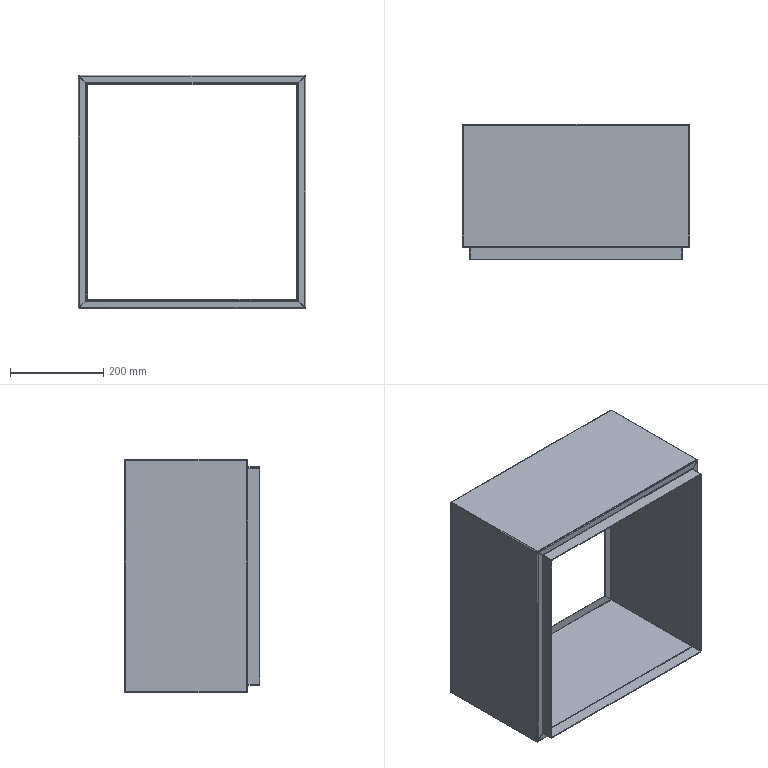Part | SolidWorks | features EdgeFlange 3, SMMiteredFlange 2, FlatPattern 1, SMBaseFlange 1, SheetMetal 1 | 1 solid | 126 faces | box 488 x 290 x 500 mm | volume 1251248 mm3 | plane 72 | cylinder 30 | spline 24 | commonest cylinder face diameters 1.473 x15 5.473 x15